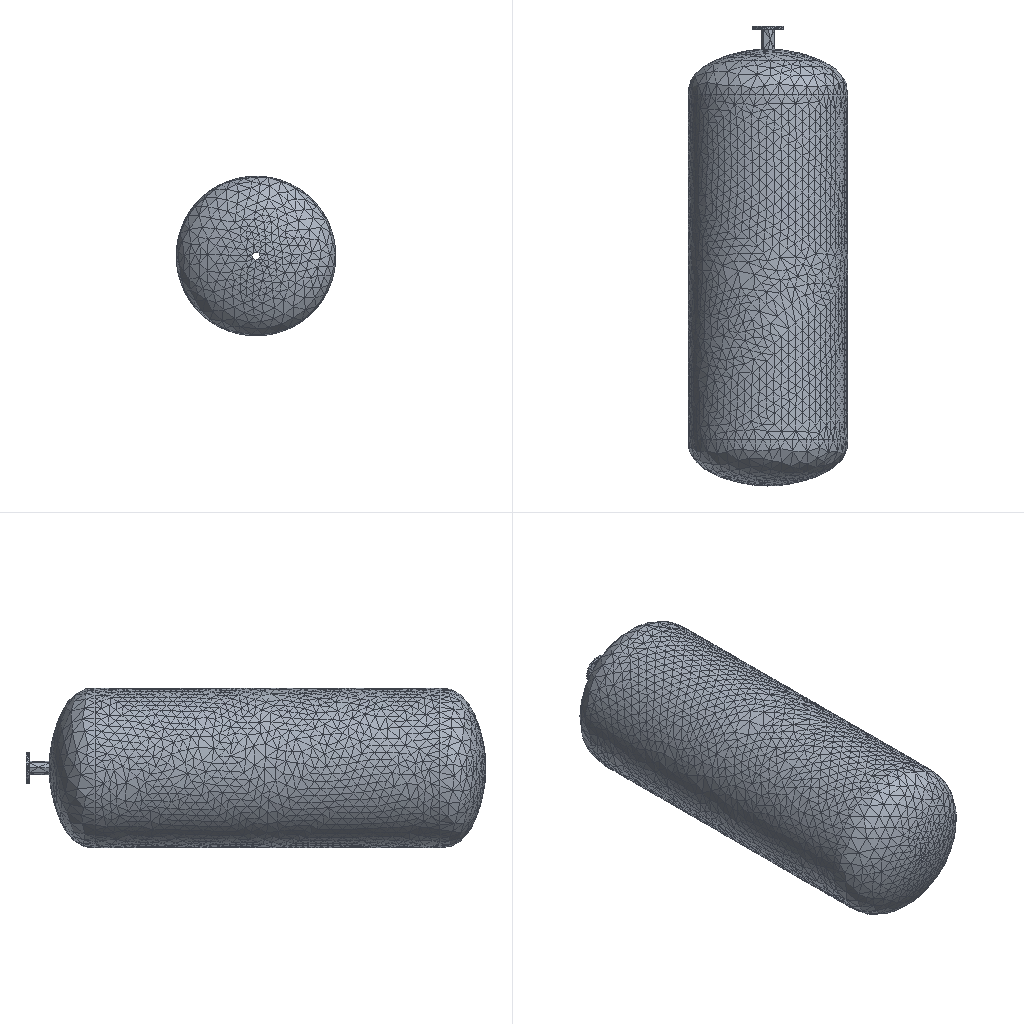Simulation study | ansys workbench
Set-up summary:
category,name,step,type,value,unit,region
solver,ansys_workbench
units,mm-N-s-tonne (MPa),,stated,"/units,MPA"
analysis,LS1,,static
load_step,LS1,LS1,static,nsubst=1; time=1
mesh,nodes,,,30530
mesh,elements,,,19029
element_type,SOLID187,,,15218
element_type,SURF154,,,3811
material,Structural Steel,,E,200000,tonne s^-2 mm^-1
material,Structural Steel,,nu,0.3
material,Structural Steel,,density,7.85e-09,tonne mm^-3
material,Structural Steel,,conductivity,60.5,tonne mm s^-3 C^-1
material,Structural Steel,,specific_heat,4.34e+08,mm^2 s^-2 C^-1
material,Structural Steel,,cte,1.2e-05,C^-1
material,Structural Steel,,permeability,10000
material,Structural Steel,,resistivity,0.00017,ohm mm
load,"Define Pressure Using Surface Effect Elements ""__""",LS1,pressure,0.5,,SURF154 #2
load,Define Force Using Surface Effect Elements,LS1,surface-effect pres face 1,-4.2073e-19,,SURF154 #3
load,Define Force Using Surface Effect Elements,LS1,surface-effect pres face 2,0.0908,,SURF154 #3
load,Define Force Using Surface Effect Elements,LS1,surface-effect pres face 3,-1.00728e-17,,SURF154 #3
bc,Fixed Supports,model,fixed,[dofs=ALL],,_FIXEDSU
named_set,_FIXEDSU,,node,1296
Ansys APDL input file, long lists of numbers shortened:
/batch
/config,noeldb,1     ! force off writing results to database
*get,_wallstrt,active,,time,wall
! ANSYS input file written by Workbench version 2022 R1
! File used for geometry attach:
/title,wbnew--____ (B5)
! ****** Begin Custom Load Command Snippet ******
/COM, ACT Extensions:
/COM,     LSDYNA, 2021.1
/COM,
! ****** End   Custom Load Command Snippet ******
*DIM,_wb_ProjectScratch_dir,string,248
_wb_ProjectScratch_dir(1) = ''
*DIM,_wb_SolverFiles_dir,string,248
_wb_SolverFiles_dir(1) = ''
*DIM,_wb_userfiles_dir,string,248
_wb_userfiles_dir(1) = ''
/com,--- Data in consistent NMM units. See Solving Units in the help system for more information.
/units,MPA
/nopr
/wb,file,start              !  signify a WB generated input file
/prep7
! Turn off shape checking because checks already performed inside WB mesher.
! See help system for more information.
SHPP,OFF,,NOWARN
/nolist
etcon,set             ! allow ANSYS to choose best KEYOP's for 180x elements, resets any applicable keyopt to MAPDL defaults
/com,*********** Nodes for the whole assembly ***********
nblock,3,,33583
(1i9,3e20.9e3)
    15339    -2.614677751E+02     1.762733227E+02     1.476989949E+02
! (30529 more lines like these left out)
-1
/wb,elem,start            !  set before creation of elements
/com,*********** Elements for Body 1 "__1" ***********
et,1,187
eblock,19,solid,,15218
(19i9)
        1        1        1        1        0        0        0        0       10        0     5617    15645    20405    20439    20431    22530    45833    22533    22532
! (30435 more lines like these left out)
-1
/wb,elem,end               !  done creating elements
/com,*********** Send User Defined Coordinate System(s) ***********
csys,0
toffst,273.15,  ! Temperature offset from absolute zero
/com,*********** Set Reference Temperature ***********
tref,22.
/wb,mat,start              !  starting to send materials
/com,*********** Send Materials ***********
Temperature = 'TEMP' ! Temperature
MP,DENS,1,7.85e-09,	! tonne mm^-3
MP,ALPX,1,1.2e-05,	! C^-1
MP,C,1,434000000,	! mm^2 s^-2 C^-1
MP,KXX,1,60.5,	! tonne mm s^-3 C^-1
MP,RSVX,1,0.00017,	! ohm mm
MP,EX,1,200000,	! tonne s^-2 mm^-1
MP,NUXY,1,0.3,
MP,MURX,1,10000,
/wb,mat,end                !  done sending materials
!************************* Model Summary ********************
!__1,	结构钢,	matid,	1
!************************* End Model Summary ********************
! get the diagonal of the bounding box. Needed later for other things
*get,_xmin,node,,mnloc,x
*get,_ymin,node,,mnloc,y
*get,_zmin,node,,mnloc,z
*get,_xmax,node,,mxloc,x
*get,_ymax,node,,mxloc,y
*get,_zmax,node,,mxloc,z
_ASMDIAG=(_xmax-_xmin)*(_xmax-_xmin)+(_ymax-_ymin)*(_ymax-_ymin)+(_zmax-_zmin)*(_zmax-_zmin)
_ASMDIAG=SQRT(_ASMDIAG)
/wb,contact,start          !  starting to send contact
/wb,contact,end            !  done creating contacts
/golist
/wb,load,start             !  starting to send loads
/com,*********** Fixed Supports ***********
CMBLOCK,_FIXEDSU,NODE,     1296
(8i10)
     15362     15363     15364     15365     15366     15367     15368     15369
! (161 more lines like these left out)
cmsel,s,_FIXEDSU
d,all,all
nsel,all
/com,*********** Define Pressure Using Surface Effect Elements "__" ***********
et,2,154
eblock,10,,,3661
(15i9)
    36147        2        2        2        0    15760    15634    18643    18643    22440    22447    18643    23167
! (3660 more lines like these left out)
-1
esel,s,type,,2
keyop,2,7,0                ! Use deformed area for application of load
esel,all
/com,*********** Define Force Using Surface Effect Elements ***********
local,12,0,0.,0.,0.,0.,0.,0.
csys,0
et,3,154
eblock,10,,,150
(15i9)
    39808        3        3        3       12    15424    15672    15467    15467    21114    21345    15467    21112
! (149 more lines like these left out)
-1
esel,s,type,,3
keyop,3,2,1                ! Apply load in local coordinate system
keyop,3,7,1                ! Use original area so load is constant in large deformation
esel,all
esel,all
/gst,on,on
fini
*get,_numnode,node,0,count
*get,_numelem,elem,0,count
*get, _MAXELEMNUM, elem, 0, NUM, MAX
*get, _MAXNODENUM, node, 0, NUM, MAX
*get, _MAXELEMTYPE, etyp, 0, NUM, MAX
*get, _MAXREALCONST, real, 0, NUM, MAX
/go
/wb,load,end               !  done creating loads
/com,--- Number of total nodes = %_numnode%
/com,--- Number of contact elements = 3811
/com,--- Number of spring elements = 0
/com,--- Number of bearing elements = 0
/com,--- Number of solid elements = 15218
/com,--- Number of condensed parts = 0
/com,--- Number of total elements = %_numelem%
*get,_wallbsol,active,,time,wall
/com,****************************************************************************
/com,*************************    SOLUTION       ********************************
/com,****************************************************************************
/solu
antype,0                   ! static analysis
_thickRatio=  0     ! Ratio of thick parts in the model
eqsl,sparse,,,,,1
cntr,print,1               ! print out contact info and also make no initial contact an error
dmpoption,emat,no             ! Don't combine emat file for DANSYS
dmpoption,esav,no             ! Don't combine esav file for DANSYS
nldiag,cont,iter           ! print out contact info each equilibrium iteration
rescontrol,,none                 ! Do not keep any restart files
/com,****************************************************
/com,******************* SOLVE FOR LS 1 OF 1 ****************
esel,s,type,,2
nsle
sf,all,pres,0.5
nsel,all
esel,all
esel,s,type,,3
nsle
sfe,all,1,pres,1,-4.20729865682867e-019
sfe,all,2,pres,1,9.08021992398707e-002
sfe,all,3,pres,1,-1.00728047446896e-017
nsel,all
esel,all
esel,all
/nopr
/gopr
nsub,1,1,1
time,1.
outres,erase
outres,all,none
outres,nsol,all,
outres,rsol,all
outres,eangl,all
outres,etmp,all
outres,veng,all
outres,strs,all,
outres,epel,all,
outres,eppl,all,
outres,cont,all,
! *********** WB SOLVE COMMAND ***********
! check interactive state
*get,ANSINTER_,active,,int
*if,ANSINTER_,ne,0,then
/eof
*endif
solve
/com *************** Write FE CONNECTORS *********
CEWRITE,file,ce,,INTE
/com,****************************************************
/com,*************** FINISHED SOLVE FOR LS 1 *************
*get,_wallasol,active,,time,wall
/nopr
*get,_numnode,node,0,count
*get,_numelem,elem,0,count
*get, _MAXELEMNUM, elem, 0, NUM, MAX
*get, _MAXNODENUM, node, 0, NUM, MAX,,,INTERNAL
*get, _MAXELEMTYPE, etyp, 0, NUM, MAX
*get, _MAXREALCONST, real, 0, NUM, MAX
/gopr
/post1
xmlo,ENCODING,ISO-8859-1
xmlo,parm
/xml,parm,xml
fini
/gopr
*get,_walldone,active,,time,wall
_preptime=(_wallbsol-_wallstrt)*3600
_solvtime=(_wallasol-_wallbsol)*3600
_posttime=(_walldone-_wallasol)*3600
_totaltim=(_walldone-_wallstrt)*3600
*get,_dlbratio,active,0,solu,dlbr
*get,_combtime,active,0,solu,comb
*get,_ssmode,active,0,solu,ssmm
*get,_ndofs,active,0,solu,ndof
*get,_sol_end_time,active,0,set,time
*if,_sol_end_time,eq,1.,then
/fclean				!clean distributed files
*endif
/com,--- Total number of nodes = %_numnode%
/com,--- Total number of elements = %_numelem%
/com,--- Element load balance ratio = %_dlbratio%
/com,--- Time to combine distributed files = %_combtime%
/com,--- Sparse memory mode = %_ssmode%
/com,--- Number of DOF = %_ndofs%
/wb,file,end               ! done with WB generated input
Results summary:
result,analyses[0].index,,,1
result,analyses[0].system,,,SYS
result,analyses[0].deck,,,deck.dat
result,analyses[0].solve_status,,,completed
result,analyses[0].analysis_type,,,static
result,analyses[0].physics,,,mechanical
result,analyses[0].unit_system,,,"NMM: mm, ton, N, s, mV, mA, degC"
result,analyses[0].n_sets,,,1
result,analyses[0].load_steps[0].set,set=1,,1
result,analyses[0].load_steps[0].time_or_freq,set=1,,1
result,analyses[0].load_steps[0].max_displacement_magnitude,set=1,,0.009875
result,analyses[0].load_steps[0].max_von_mises_nodal,set=1,,14.359
result,analyses[0].load_steps[0].reaction_force_sum_xyz[1],set=1,,-7.34502e-09
result,analyses[0].load_steps[0].reaction_force_sum_xyz[2],set=1,,-99.999
result,analyses[0].load_steps[0].reaction_force_sum_xyz[3],set=1,,8.17788e-09